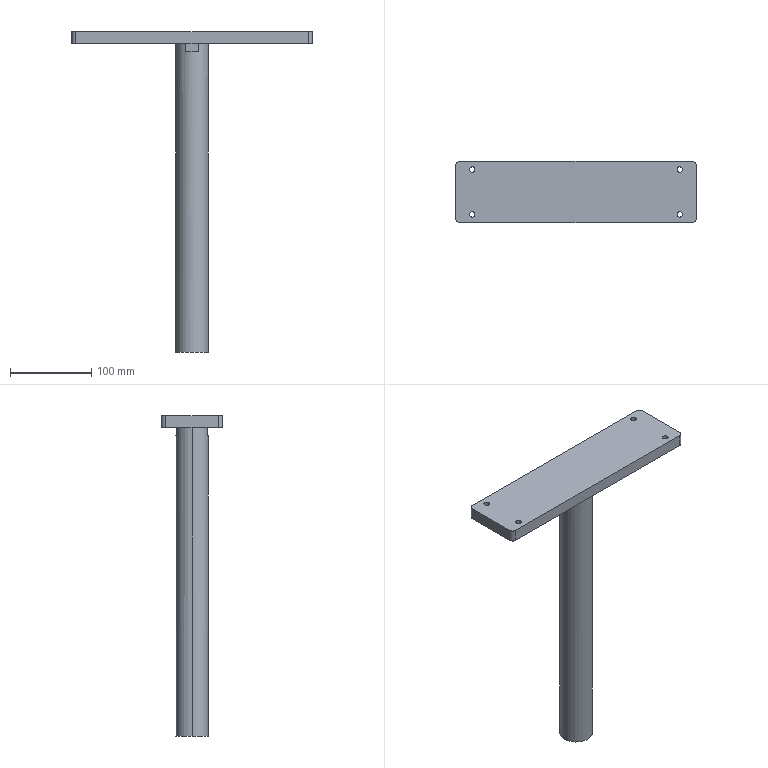Part | STEP file | Electric cylinder assembly 1 | 1 solid | 25 faces | box 295 x 75 x 394 mm | volume 805333 mm3 | cylinder 14 | plane 11 | commonest cylinder face diameters 6.8 x8 10 x4 40 x2
STEP:
#1=CARTESIAN_POINT('',(15.373,-48.431,607.5));
#2=VERTEX_POINT('',#1);
#3=CARTESIAN_POINT('',(2.972,-29.931,607.5));
#4=VERTEX_POINT('',#3);
#5=CARTESIAN_POINT('',(-4.627,-48.431,607.5));
#6=DIRECTION('',(0.,0.,1.));
#7=DIRECTION('',(1.,0.,0.));
#8=AXIS2_PLACEMENT_3D('',#5,#6,#7);
#9=CIRCLE('',#8,20.);
#10=EDGE_CURVE('',#2,#4,#9,.T.);
#11=ORIENTED_EDGE('',*,*,#10,.F.);
#12=CARTESIAN_POINT('',(15.373,-48.431,228.5));
#13=VERTEX_POINT('',#12);
#14=CARTESIAN_POINT('',(15.373,-48.431,580.5));
#15=DIRECTION('',(0.,0.,-1.));
#16=VECTOR('',#15,1000.);
#17=LINE('',#14,#16);
#18=EDGE_CURVE('',#2,#13,#17,.T.);
#19=ORIENTED_EDGE('',*,*,#18,.T.);
#20=CARTESIAN_POINT('',(-24.627,-48.431,228.5));
#21=VERTEX_POINT('',#20);
#22=CARTESIAN_POINT('',(-4.627,-48.431,228.5));
#23=DIRECTION('',(0.,0.,-1.));
#24=DIRECTION('',(-1.,0.,0.));
#25=AXIS2_PLACEMENT_3D('',#22,#23,#24);
#26=CIRCLE('',#25,20.);
#27=EDGE_CURVE('',#21,#13,#26,.T.);
#28=ORIENTED_EDGE('',*,*,#27,.F.);
#29=CARTESIAN_POINT('',(-24.627,-48.431,607.5));
#30=VERTEX_POINT('',#29);
#31=CARTESIAN_POINT('',(-24.627,-48.431,580.5));
#32=DIRECTION('',(0.,0.,-1.));
#33=VECTOR('',#32,1000.);
#34=LINE('',#31,#33);
#35=EDGE_CURVE('',#30,#21,#34,.T.);
#36=ORIENTED_EDGE('',*,*,#35,.F.);
#37=CARTESIAN_POINT('',(-12.227,-29.931,607.5));
#38=VERTEX_POINT('',#37);
#39=CARTESIAN_POINT('',(-4.627,-48.431,607.5));
#40=DIRECTION('',(0.,0.,1.));
#41=DIRECTION('',(1.,0.,0.));
#42=AXIS2_PLACEMENT_3D('',#39,#40,#41);
#43=CIRCLE('',#42,20.);
#44=EDGE_CURVE('',#38,#30,#43,.T.);
#45=ORIENTED_EDGE('',*,*,#44,.F.);
#46=CARTESIAN_POINT('',(-12.227,-29.931,597.5));
#47=VERTEX_POINT('',#46);
#48=CARTESIAN_POINT('',(-12.227,-29.931,607.5));
#49=DIRECTION('',(0.,0.,-1.));
#50=VECTOR('',#49,1000.);
#51=LINE('',#48,#50);
#52=EDGE_CURVE('',#38,#47,#51,.T.);
#53=ORIENTED_EDGE('',*,*,#52,.T.);
#54=CARTESIAN_POINT('',(2.972,-29.931,597.5));
#55=VERTEX_POINT('',#54);
#56=CARTESIAN_POINT('',(-4.627,-48.431,597.5));
#57=DIRECTION('',(0.,0.,-1.));
#58=DIRECTION('',(-1.,0.,0.));
#59=AXIS2_PLACEMENT_3D('',#56,#57,#58);
#60=CIRCLE('',#59,20.);
#61=EDGE_CURVE('',#47,#55,#60,.T.);
#62=ORIENTED_EDGE('',*,*,#61,.T.);
#63=CARTESIAN_POINT('',(2.972,-29.931,607.5));
#64=DIRECTION('',(0.,0.,1.));
#65=VECTOR('',#64,1000.);
#66=LINE('',#63,#65);
#67=EDGE_CURVE('',#55,#4,#66,.T.);
#68=ORIENTED_EDGE('',*,*,#67,.T.);
#69=EDGE_LOOP('',(#11,#19,#28,#36,#45,#53,#62,#68));
#70=FACE_OUTER_BOUND('',#69,.T.);
#71=CARTESIAN_POINT('',(-4.627,-48.431,580.5));
#72=DIRECTION('',(0.,0.,-1.));
#73=DIRECTION('',(-1.,0.,0.));
#74=AXIS2_PLACEMENT_3D('',#71,#72,#73);
#75=CYLINDRICAL_SURFACE('',#74,20.);
#76=ADVANCED_FACE('',(#70),#75,.T.);
#77=CARTESIAN_POINT('',(137.873,-85.931,622.5));
#78=VERTEX_POINT('',#77);
#79=CARTESIAN_POINT('',(142.873,-80.931,622.5));
#80=VERTEX_POINT('',#79);
#81=CARTESIAN_POINT('',(137.873,-80.931,622.5));
#82=DIRECTION('',(0.,0.,1.));
#83=DIRECTION('',(1.,0.,0.));
#84=AXIS2_PLACEMENT_3D('',#81,#82,#83);
#85=CIRCLE('',#84,5.);
#86=EDGE_CURVE('',#78,#80,#85,.T.);
#87=ORIENTED_EDGE('',*,*,#86,.F.);
#88=CARTESIAN_POINT('',(137.873,-85.931,607.5));
#89=VERTEX_POINT('',#88);
#90=CARTESIAN_POINT('',(137.873,-85.931,622.5));
#91=DIRECTION('',(0.,0.,1.));
#92=VECTOR('',#91,1000.);
#93=LINE('',#90,#92);
#94=EDGE_CURVE('',#89,#78,#93,.T.);
#95=ORIENTED_EDGE('',*,*,#94,.F.);
#96=CARTESIAN_POINT('',(142.873,-80.931,607.5));
#97=VERTEX_POINT('',#96);
#98=CARTESIAN_POINT('',(137.873,-80.931,607.5));
#99=DIRECTION('',(0.,0.,-1.));
#100=DIRECTION('',(1.,0.,0.));
#101=AXIS2_PLACEMENT_3D('',#98,#99,#100);
#102=CIRCLE('',#101,5.);
#103=EDGE_CURVE('',#97,#89,#102,.T.);
#104=ORIENTED_EDGE('',*,*,#103,.F.);
#105=CARTESIAN_POINT('',(142.873,-80.931,622.5));
#106=DIRECTION('',(0.,0.,-1.));
#107=VECTOR('',#106,1000.);
#108=LINE('',#105,#107);
#109=EDGE_CURVE('',#80,#97,#108,.T.);
#110=ORIENTED_EDGE('',*,*,#109,.F.);
#111=EDGE_LOOP('',(#87,#95,#104,#110));
#112=FACE_OUTER_BOUND('',#111,.T.);
#113=CARTESIAN_POINT('',(137.873,-80.931,622.5));
#114=DIRECTION('',(0.,0.,-1.));
#115=DIRECTION('',(-1.,0.,0.));
#116=AXIS2_PLACEMENT_3D('',#113,#114,#115);
#117=CYLINDRICAL_SURFACE('',#116,5.);
#118=ADVANCED_FACE('',(#112),#117,.T.);
#119=CARTESIAN_POINT('',(142.873,-15.931,607.5));
#120=VERTEX_POINT('',#119);
#121=CARTESIAN_POINT('',(142.873,-10.931,607.5));
#122=DIRECTION('',(0.,1.,0.));
#123=VECTOR('',#122,1000.);
#124=LINE('',#121,#123);
#125=EDGE_CURVE('',#97,#120,#124,.T.);
#126=ORIENTED_EDGE('',*,*,#125,.T.);
#127=CARTESIAN_POINT('',(142.873,-15.931,622.5));
#128=VERTEX_POINT('',#127);
#129=CARTESIAN_POINT('',(142.873,-15.931,622.5));
#130=DIRECTION('',(0.,0.,1.));
#131=VECTOR('',#130,1000.);
#132=LINE('',#129,#131);
#133=EDGE_CURVE('',#120,#128,#132,.T.);
#134=ORIENTED_EDGE('',*,*,#133,.T.);
#135=CARTESIAN_POINT('',(142.873,-10.931,622.5));
#136=DIRECTION('',(0.,1.,0.));
#137=VECTOR('',#136,1000.);
#138=LINE('',#135,#137);
#139=EDGE_CURVE('',#80,#128,#138,.T.);
#140=ORIENTED_EDGE('',*,*,#139,.F.);
#141=ORIENTED_EDGE('',*,*,#109,.T.);
#142=EDGE_LOOP('',(#126,#134,#140,#141));
#143=FACE_OUTER_BOUND('',#142,.T.);
#144=CARTESIAN_POINT('',(142.873,-10.931,622.5));
#145=DIRECTION('',(-1.,0.,0.));
#146=DIRECTION('',(0.,0.,1.));
#147=AXIS2_PLACEMENT_3D('',#144,#145,#146);
#148=PLANE('',#147);
#149=ADVANCED_FACE('',(#143),#148,.F.);
#150=CARTESIAN_POINT('',(137.873,-10.931,622.5));
#151=VERTEX_POINT('',#150);
#152=CARTESIAN_POINT('',(137.873,-15.931,622.5));
#153=DIRECTION('',(0.,0.,1.));
#154=DIRECTION('',(1.,0.,0.));
#155=AXIS2_PLACEMENT_3D('',#152,#153,#154);
#156=CIRCLE('',#155,5.);
#157=EDGE_CURVE('',#128,#151,#156,.T.);
#158=ORIENTED_EDGE('',*,*,#157,.F.);
#159=ORIENTED_EDGE('',*,*,#133,.F.);
#160=CARTESIAN_POINT('',(137.873,-10.931,607.5));
#161=VERTEX_POINT('',#160);
#162=CARTESIAN_POINT('',(137.873,-15.931,607.5));
#163=DIRECTION('',(0.,0.,-1.));
#164=DIRECTION('',(1.,0.,0.));
#165=AXIS2_PLACEMENT_3D('',#162,#163,#164);
#166=CIRCLE('',#165,5.);
#167=EDGE_CURVE('',#161,#120,#166,.T.);
#168=ORIENTED_EDGE('',*,*,#167,.F.);
#169=CARTESIAN_POINT('',(137.873,-10.931,622.5));
#170=DIRECTION('',(0.,0.,-1.));
#171=VECTOR('',#170,1000.);
#172=LINE('',#169,#171);
#173=EDGE_CURVE('',#151,#161,#172,.T.);
#174=ORIENTED_EDGE('',*,*,#173,.F.);
#175=EDGE_LOOP('',(#158,#159,#168,#174));
#176=FACE_OUTER_BOUND('',#175,.T.);
#177=CARTESIAN_POINT('',(137.873,-15.931,622.5));
#178=DIRECTION('',(0.,0.,-1.));
#179=DIRECTION('',(-1.,0.,0.));
#180=AXIS2_PLACEMENT_3D('',#177,#178,#179);
#181=CYLINDRICAL_SURFACE('',#180,5.);
#182=ADVANCED_FACE('',(#176),#181,.T.);
#183=CARTESIAN_POINT('',(119.473,-20.931,607.5));
#184=VERTEX_POINT('',#183);
#185=CARTESIAN_POINT('',(126.273,-20.931,607.5));
#186=VERTEX_POINT('',#185);
#187=CARTESIAN_POINT('',(122.873,-20.931,607.5));
#188=DIRECTION('',(0.,0.,1.));
#189=DIRECTION('',(1.,0.,0.));
#190=AXIS2_PLACEMENT_3D('',#187,#188,#189);
#191=CIRCLE('',#190,3.4);
#192=EDGE_CURVE('',#184,#186,#191,.T.);
#193=ORIENTED_EDGE('',*,*,#192,.F.);
#194=CARTESIAN_POINT('',(119.473,-20.931,622.5));
#195=VERTEX_POINT('',#194);
#196=CARTESIAN_POINT('',(119.473,-20.931,622.5));
#197=DIRECTION('',(0.,0.,1.));
#198=VECTOR('',#197,1000.);
#199=LINE('',#196,#198);
#200=EDGE_CURVE('',#184,#195,#199,.T.);
#201=ORIENTED_EDGE('',*,*,#200,.T.);
#202=CARTESIAN_POINT('',(126.273,-20.931,622.5));
#203=VERTEX_POINT('',#202);
#204=CARTESIAN_POINT('',(122.873,-20.931,622.5));
#205=DIRECTION('',(0.,0.,1.));
#206=DIRECTION('',(1.,0.,0.));
#207=AXIS2_PLACEMENT_3D('',#204,#205,#206);
#208=CIRCLE('',#207,3.4);
#209=EDGE_CURVE('',#195,#203,#208,.T.);
#210=ORIENTED_EDGE('',*,*,#209,.T.);
#211=CARTESIAN_POINT('',(126.273,-20.931,622.5));
#212=DIRECTION('',(0.,0.,1.));
#213=VECTOR('',#212,1000.);
#214=LINE('',#211,#213);
#215=EDGE_CURVE('',#186,#203,#214,.T.);
#216=ORIENTED_EDGE('',*,*,#215,.F.);
#217=EDGE_LOOP('',(#193,#201,#210,#216));
#218=FACE_OUTER_BOUND('',#217,.T.);
#219=CARTESIAN_POINT('',(122.873,-20.931,622.5));
#220=DIRECTION('',(0.,0.,1.));
#221=DIRECTION('',(1.,0.,0.));
#222=AXIS2_PLACEMENT_3D('',#219,#220,#221);
#223=CYLINDRICAL_SURFACE('',#222,3.4);
#224=ADVANCED_FACE('',(#218),#223,.F.);
#225=ORIENTED_EDGE('',*,*,#200,.F.);
#226=CARTESIAN_POINT('',(122.873,-20.931,607.5));
#227=DIRECTION('',(0.,0.,1.));
#228=DIRECTION('',(1.,0.,0.));
#229=AXIS2_PLACEMENT_3D('',#226,#227,#228);
#230=CIRCLE('',#229,3.4);
#231=EDGE_CURVE('',#186,#184,#230,.T.);
#232=ORIENTED_EDGE('',*,*,#231,.F.);
#233=ORIENTED_EDGE('',*,*,#215,.T.);
#234=CARTESIAN_POINT('',(122.873,-20.931,622.5));
#235=DIRECTION('',(0.,0.,1.));
#236=DIRECTION('',(1.,0.,0.));
#237=AXIS2_PLACEMENT_3D('',#234,#235,#236);
#238=CIRCLE('',#237,3.4);
#239=EDGE_CURVE('',#203,#195,#238,.T.);
#240=ORIENTED_EDGE('',*,*,#239,.T.);
#241=EDGE_LOOP('',(#225,#232,#233,#240));
#242=FACE_OUTER_BOUND('',#241,.T.);
#243=CARTESIAN_POINT('',(122.873,-20.931,622.5));
#244=DIRECTION('',(0.,0.,1.));
#245=DIRECTION('',(1.,0.,0.));
#246=AXIS2_PLACEMENT_3D('',#243,#244,#245);
#247=CYLINDRICAL_SURFACE('',#246,3.4);
#248=ADVANCED_FACE('',(#242),#247,.F.);
#249=CARTESIAN_POINT('',(119.473,-75.931,607.5));
#250=VERTEX_POINT('',#249);
#251=CARTESIAN_POINT('',(126.273,-75.931,607.5));
#252=VERTEX_POINT('',#251);
#253=CARTESIAN_POINT('',(122.873,-75.931,607.5));
#254=DIRECTION('',(0.,0.,1.));
#255=DIRECTION('',(1.,0.,0.));
#256=AXIS2_PLACEMENT_3D('',#253,#254,#255);
#257=CIRCLE('',#256,3.4);
#258=EDGE_CURVE('',#250,#252,#257,.T.);
#259=ORIENTED_EDGE('',*,*,#258,.F.);
#260=CARTESIAN_POINT('',(119.473,-75.931,622.5));
#261=VERTEX_POINT('',#260);
#262=CARTESIAN_POINT('',(119.473,-75.931,622.5));
#263=DIRECTION('',(0.,0.,1.));
#264=VECTOR('',#263,1000.);
#265=LINE('',#262,#264);
#266=EDGE_CURVE('',#250,#261,#265,.T.);
#267=ORIENTED_EDGE('',*,*,#266,.T.);
#268=CARTESIAN_POINT('',(126.273,-75.931,622.5));
#269=VERTEX_POINT('',#268);
#270=CARTESIAN_POINT('',(122.873,-75.931,622.5));
#271=DIRECTION('',(0.,0.,1.));
#272=DIRECTION('',(1.,0.,0.));
#273=AXIS2_PLACEMENT_3D('',#270,#271,#272);
#274=CIRCLE('',#273,3.4);
#275=EDGE_CURVE('',#261,#269,#274,.T.);
#276=ORIENTED_EDGE('',*,*,#275,.T.);
#277=CARTESIAN_POINT('',(126.273,-75.931,622.5));
#278=DIRECTION('',(0.,0.,1.));
#279=VECTOR('',#278,1000.);
#280=LINE('',#277,#279);
#281=EDGE_CURVE('',#252,#269,#280,.T.);
#282=ORIENTED_EDGE('',*,*,#281,.F.);
#283=EDGE_LOOP('',(#259,#267,#276,#282));
#284=FACE_OUTER_BOUND('',#283,.T.);
#285=CARTESIAN_POINT('',(122.873,-75.931,622.5));
#286=DIRECTION('',(0.,0.,1.));
#287=DIRECTION('',(1.,0.,0.));
#288=AXIS2_PLACEMENT_3D('',#285,#286,#287);
#289=CYLINDRICAL_SURFACE('',#288,3.4);
#290=ADVANCED_FACE('',(#284),#289,.F.);
#291=ORIENTED_EDGE('',*,*,#266,.F.);
#292=CARTESIAN_POINT('',(122.873,-75.931,607.5));
#293=DIRECTION('',(0.,0.,1.));
#294=DIRECTION('',(1.,0.,0.));
#295=AXIS2_PLACEMENT_3D('',#292,#293,#294);
#296=CIRCLE('',#295,3.4);
#297=EDGE_CURVE('',#252,#250,#296,.T.);
#298=ORIENTED_EDGE('',*,*,#297,.F.);
#299=ORIENTED_EDGE('',*,*,#281,.T.);
#300=CARTESIAN_POINT('',(122.873,-75.931,622.5));
#301=DIRECTION('',(0.,0.,1.));
#302=DIRECTION('',(1.,0.,0.));
#303=AXIS2_PLACEMENT_3D('',#300,#301,#302);
#304=CIRCLE('',#303,3.4);
#305=EDGE_CURVE('',#269,#261,#304,.T.);
#306=ORIENTED_EDGE('',*,*,#305,.T.);
#307=EDGE_LOOP('',(#291,#298,#299,#306));
#308=FACE_OUTER_BOUND('',#307,.T.);
#309=CARTESIAN_POINT('',(122.873,-75.931,622.5));
#310=DIRECTION('',(0.,0.,1.));
#311=DIRECTION('',(1.,0.,0.));
#312=AXIS2_PLACEMENT_3D('',#309,#310,#311);
#313=CYLINDRICAL_SURFACE('',#312,3.4);
#314=ADVANCED_FACE('',(#308),#313,.F.);
#315=ORIENTED_EDGE('',*,*,#297,.T.);
#316=ORIENTED_EDGE('',*,*,#258,.T.);
#317=EDGE_LOOP('',(#315,#316));
#318=FACE_BOUND('',#317,.T.);
#319=ORIENTED_EDGE('',*,*,#231,.T.);
#320=ORIENTED_EDGE('',*,*,#192,.T.);
#321=EDGE_LOOP('',(#319,#320));
#322=FACE_BOUND('',#321,.T.);
#323=CARTESIAN_POINT('',(-147.127,-85.931,607.5));
#324=VERTEX_POINT('',#323);
#325=CARTESIAN_POINT('',(-12.127,-85.931,607.5));
#326=DIRECTION('',(1.,0.,0.));
#327=VECTOR('',#326,1000.);
#328=LINE('',#325,#327);
#329=EDGE_CURVE('',#324,#89,#328,.T.);
#330=ORIENTED_EDGE('',*,*,#329,.F.);
#331=CARTESIAN_POINT('',(-152.127,-80.931,607.5));
#332=VERTEX_POINT('',#331);
#333=CARTESIAN_POINT('',(-147.127,-80.931,607.5));
#334=DIRECTION('',(0.,0.,-1.));
#335=DIRECTION('',(1.,0.,0.));
#336=AXIS2_PLACEMENT_3D('',#333,#334,#335);
#337=CIRCLE('',#336,5.);
#338=EDGE_CURVE('',#324,#332,#337,.T.);
#339=ORIENTED_EDGE('',*,*,#338,.T.);
#340=CARTESIAN_POINT('',(-152.127,-15.931,607.5));
#341=VERTEX_POINT('',#340);
#342=CARTESIAN_POINT('',(-152.127,-10.931,607.5));
#343=DIRECTION('',(0.,-1.,0.));
#344=VECTOR('',#343,1000.);
#345=LINE('',#342,#344);
#346=EDGE_CURVE('',#341,#332,#345,.T.);
#347=ORIENTED_EDGE('',*,*,#346,.F.);
#348=CARTESIAN_POINT('',(-147.127,-10.931,607.5));
#349=VERTEX_POINT('',#348);
#350=CARTESIAN_POINT('',(-147.127,-15.931,607.5));
#351=DIRECTION('',(0.,0.,-1.));
#352=DIRECTION('',(1.,0.,0.));
#353=AXIS2_PLACEMENT_3D('',#350,#351,#352);
#354=CIRCLE('',#353,5.);
#355=EDGE_CURVE('',#341,#349,#354,.T.);
#356=ORIENTED_EDGE('',*,*,#355,.T.);
#357=CARTESIAN_POINT('',(-12.127,-10.931,607.5));
#358=DIRECTION('',(-1.,0.,0.));
#359=VECTOR('',#358,1000.);
#360=LINE('',#357,#359);
#361=EDGE_CURVE('',#161,#349,#360,.T.);
#362=ORIENTED_EDGE('',*,*,#361,.F.);
#363=ORIENTED_EDGE('',*,*,#167,.T.);
#364=ORIENTED_EDGE('',*,*,#125,.F.);
#365=ORIENTED_EDGE('',*,*,#103,.T.);
#366=EDGE_LOOP('',(#330,#339,#347,#356,#362,#363,#364,#365));
#367=FACE_OUTER_BOUND('',#366,.T.);
#368=CARTESIAN_POINT('',(2.972,-66.931,607.5));
#369=VERTEX_POINT('',#368);
#370=CARTESIAN_POINT('',(-4.627,-48.431,607.5));
#371=DIRECTION('',(0.,0.,1.));
#372=DIRECTION('',(1.,0.,0.));
#373=AXIS2_PLACEMENT_3D('',#370,#371,#372);
#374=CIRCLE('',#373,20.);
#375=EDGE_CURVE('',#369,#2,#374,.T.);
#376=ORIENTED_EDGE('',*,*,#375,.T.);
#377=ORIENTED_EDGE('',*,*,#10,.T.);
#378=CARTESIAN_POINT('',(-4.627,-29.931,607.5));
#379=DIRECTION('',(1.,0.,0.));
#380=VECTOR('',#379,1000.);
#381=LINE('',#378,#380);
#382=EDGE_CURVE('',#38,#4,#381,.T.);
#383=ORIENTED_EDGE('',*,*,#382,.F.);
#384=ORIENTED_EDGE('',*,*,#44,.T.);
#385=CARTESIAN_POINT('',(-12.227,-66.931,607.5));
#386=VERTEX_POINT('',#385);
#387=CARTESIAN_POINT('',(-4.627,-48.431,607.5));
#388=DIRECTION('',(0.,0.,1.));
#389=DIRECTION('',(1.,0.,0.));
#390=AXIS2_PLACEMENT_3D('',#387,#388,#389);
#391=CIRCLE('',#390,20.);
#392=EDGE_CURVE('',#30,#386,#391,.T.);
#393=ORIENTED_EDGE('',*,*,#392,.T.);
#394=CARTESIAN_POINT('',(-4.627,-66.931,607.5));
#395=DIRECTION('',(-1.,0.,0.));
#396=VECTOR('',#395,1000.);
#397=LINE('',#394,#396);
#398=EDGE_CURVE('',#369,#386,#397,.T.);
#399=ORIENTED_EDGE('',*,*,#398,.F.);
#400=EDGE_LOOP('',(#376,#377,#383,#384,#393,#399));
#401=FACE_BOUND('',#400,.T.);
#402=CARTESIAN_POINT('',(-128.727,-75.931,607.5));
#403=VERTEX_POINT('',#402);
#404=CARTESIAN_POINT('',(-135.527,-75.931,607.5));
#405=VERTEX_POINT('',#404);
#406=CARTESIAN_POINT('',(-132.127,-75.931,607.5));
#407=DIRECTION('',(0.,0.,1.));
#408=DIRECTION('',(1.,0.,0.));
#409=AXIS2_PLACEMENT_3D('',#406,#407,#408);
#410=CIRCLE('',#409,3.4);
#411=EDGE_CURVE('',#403,#405,#410,.T.);
#412=ORIENTED_EDGE('',*,*,#411,.T.);
#413=CARTESIAN_POINT('',(-132.127,-75.931,607.5));
#414=DIRECTION('',(0.,0.,1.));
#415=DIRECTION('',(1.,0.,0.));
#416=AXIS2_PLACEMENT_3D('',#413,#414,#415);
#417=CIRCLE('',#416,3.4);
#418=EDGE_CURVE('',#405,#403,#417,.T.);
#419=ORIENTED_EDGE('',*,*,#418,.T.);
#420=EDGE_LOOP('',(#412,#419));
#421=FACE_BOUND('',#420,.T.);
#422=CARTESIAN_POINT('',(-128.727,-20.931,607.5));
#423=VERTEX_POINT('',#422);
#424=CARTESIAN_POINT('',(-135.527,-20.931,607.5));
#425=VERTEX_POINT('',#424);
#426=CARTESIAN_POINT('',(-132.127,-20.931,607.5));
#427=DIRECTION('',(0.,0.,1.));
#428=DIRECTION('',(1.,0.,0.));
#429=AXIS2_PLACEMENT_3D('',#426,#427,#428);
#430=CIRCLE('',#429,3.4);
#431=EDGE_CURVE('',#423,#425,#430,.T.);
#432=ORIENTED_EDGE('',*,*,#431,.T.);
#433=CARTESIAN_POINT('',(-132.127,-20.931,607.5));
#434=DIRECTION('',(0.,0.,1.));
#435=DIRECTION('',(1.,0.,0.));
#436=AXIS2_PLACEMENT_3D('',#433,#434,#435);
#437=CIRCLE('',#436,3.4);
#438=EDGE_CURVE('',#425,#423,#437,.T.);
#439=ORIENTED_EDGE('',*,*,#438,.T.);
#440=EDGE_LOOP('',(#432,#439));
#441=FACE_BOUND('',#440,.T.);
#442=CARTESIAN_POINT('',(65.373,-48.431,607.5));
#443=DIRECTION('',(0.,0.,1.));
#444=DIRECTION('',(1.,0.,0.));
#445=AXIS2_PLACEMENT_3D('',#442,#443,#444);
#446=PLANE('',#445);
#447=ADVANCED_FACE('',(#318,#322,#367,#401,#421,#441),#446,.F.);
#448=ORIENTED_EDGE('',*,*,#361,.T.);
#449=CARTESIAN_POINT('',(-147.127,-10.931,622.5));
#450=VERTEX_POINT('',#449);
#451=CARTESIAN_POINT('',(-147.127,-10.931,622.5));
#452=DIRECTION('',(0.,0.,1.));
#453=VECTOR('',#452,1000.);
#454=LINE('',#451,#453);
#455=EDGE_CURVE('',#349,#450,#454,.T.);
#456=ORIENTED_EDGE('',*,*,#455,.T.);
#457=CARTESIAN_POINT('',(-12.127,-10.931,622.5));
#458=DIRECTION('',(-1.,0.,0.));
#459=VECTOR('',#458,1000.);
#460=LINE('',#457,#459);
#461=EDGE_CURVE('',#151,#450,#460,.T.);
#462=ORIENTED_EDGE('',*,*,#461,.F.);
#463=ORIENTED_EDGE('',*,*,#173,.T.);
#464=EDGE_LOOP('',(#448,#456,#462,#463));
#465=FACE_OUTER_BOUND('',#464,.T.);
#466=CARTESIAN_POINT('',(-12.127,-10.931,622.5));
#467=DIRECTION('',(0.,-1.,0.));
#468=DIRECTION('',(0.,0.,-1.));
#469=AXIS2_PLACEMENT_3D('',#466,#467,#468);
#470=PLANE('',#469);
#471=ADVANCED_FACE('',(#465),#470,.F.);
#472=CARTESIAN_POINT('',(-147.127,-85.931,622.5));
#473=VERTEX_POINT('',#472);
#474=CARTESIAN_POINT('',(-12.127,-85.931,622.5));
#475=DIRECTION('',(1.,0.,0.));
#476=VECTOR('',#475,1000.);
#477=LINE('',#474,#476);
#478=EDGE_CURVE('',#473,#78,#477,.T.);
#479=ORIENTED_EDGE('',*,*,#478,.F.);
#480=CARTESIAN_POINT('',(-147.127,-85.931,622.5));
#481=DIRECTION('',(0.,0.,-1.));
#482=VECTOR('',#481,1000.);
#483=LINE('',#480,#482);
#484=EDGE_CURVE('',#473,#324,#483,.T.);
#485=ORIENTED_EDGE('',*,*,#484,.T.);
#486=ORIENTED_EDGE('',*,*,#329,.T.);
#487=ORIENTED_EDGE('',*,*,#94,.T.);
#488=EDGE_LOOP('',(#479,#485,#486,#487));
#489=FACE_OUTER_BOUND('',#488,.T.);
#490=CARTESIAN_POINT('',(-12.127,-85.931,622.5));
#491=DIRECTION('',(0.,1.,0.));
#492=DIRECTION('',(1.,0.,0.));
#493=AXIS2_PLACEMENT_3D('',#490,#491,#492);
#494=PLANE('',#493);
#495=ADVANCED_FACE('',(#489),#494,.F.);
#496=ORIENTED_EDGE('',*,*,#461,.T.);
#497=CARTESIAN_POINT('',(-152.127,-15.931,622.5));
#498=VERTEX_POINT('',#497);
#499=CARTESIAN_POINT('',(-147.127,-15.931,622.5));
#500=DIRECTION('',(0.,0.,1.));
#501=DIRECTION('',(1.,0.,0.));
#502=AXIS2_PLACEMENT_3D('',#499,#500,#501);
#503=CIRCLE('',#502,5.);
#504=EDGE_CURVE('',#450,#498,#503,.T.);
#505=ORIENTED_EDGE('',*,*,#504,.T.);
#506=CARTESIAN_POINT('',(-152.127,-80.931,622.5));
#507=VERTEX_POINT('',#506);
#508=CARTESIAN_POINT('',(-152.127,-10.931,622.5));
#509=DIRECTION('',(0.,-1.,0.));
#510=VECTOR('',#509,1000.);
#511=LINE('',#508,#510);
#512=EDGE_CURVE('',#498,#507,#511,.T.);
#513=ORIENTED_EDGE('',*,*,#512,.T.);
#514=CARTESIAN_POINT('',(-147.127,-80.931,622.5));
#515=DIRECTION('',(0.,0.,1.));
#516=DIRECTION('',(1.,0.,0.));
#517=AXIS2_PLACEMENT_3D('',#514,#515,#516);
#518=CIRCLE('',#517,5.);
#519=EDGE_CURVE('',#507,#473,#518,.T.);
#520=ORIENTED_EDGE('',*,*,#519,.T.);
#521=ORIENTED_EDGE('',*,*,#478,.T.);
#522=ORIENTED_EDGE('',*,*,#86,.T.);
#523=ORIENTED_EDGE('',*,*,#139,.T.);
#524=ORIENTED_EDGE('',*,*,#157,.T.);
#525=EDGE_LOOP('',(#496,#505,#513,#520,#521,#522,#523,#524));
#526=FACE_OUTER_BOUND('',#525,.T.);
#527=ORIENTED_EDGE('',*,*,#305,.F.);
#528=ORIENTED_EDGE('',*,*,#275,.F.);
#529=EDGE_LOOP('',(#527,#528));
#530=FACE_BOUND('',#529,.T.);
#531=ORIENTED_EDGE('',*,*,#239,.F.);
#532=ORIENTED_EDGE('',*,*,#209,.F.);
#533=EDGE_LOOP('',(#531,#532));
#534=FACE_BOUND('',#533,.T.);
#535=CARTESIAN_POINT('',(-128.727,-20.931,622.5));
#536=VERTEX_POINT('',#535);
#537=CARTESIAN_POINT('',(-135.527,-20.931,622.5));
#538=VERTEX_POINT('',#537);
#539=CARTESIAN_POINT('',(-132.127,-20.931,622.5));
#540=DIRECTION('',(0.,0.,1.));
#541=DIRECTION('',(1.,0.,0.));
#542=AXIS2_PLACEMENT_3D('',#539,#540,#541);
#543=CIRCLE('',#542,3.4);
#544=EDGE_CURVE('',#536,#538,#543,.T.);
#545=ORIENTED_EDGE('',*,*,#544,.F.);
#546=CARTESIAN_POINT('',(-132.127,-20.931,622.5));
#547=DIRECTION('',(0.,0.,1.));
#548=DIRECTION('',(1.,0.,0.));
#549=AXIS2_PLACEMENT_3D('',#546,#547,#548);
#550=CIRCLE('',#549,3.4);
#551=EDGE_CURVE('',#538,#536,#550,.T.);
#552=ORIENTED_EDGE('',*,*,#551,.F.);
#553=EDGE_LOOP('',(#545,#552));
#554=FACE_BOUND('',#553,.T.);
#555=CARTESIAN_POINT('',(-128.727,-75.931,622.5));
#556=VERTEX_POINT('',#555);
#557=CARTESIAN_POINT('',(-135.527,-75.931,622.5));
#558=VERTEX_POINT('',#557);
#559=CARTESIAN_POINT('',(-132.127,-75.931,622.5));
#560=DIRECTION('',(0.,0.,1.));
#561=DIRECTION('',(1.,0.,0.));
#562=AXIS2_PLACEMENT_3D('',#559,#560,#561);
#563=CIRCLE('',#562,3.4);
#564=EDGE_CURVE('',#556,#558,#563,.T.);
#565=ORIENTED_EDGE('',*,*,#564,.F.);
#566=CARTESIAN_POINT('',(-132.127,-75.931,622.5));
#567=DIRECTION('',(0.,0.,1.));
#568=DIRECTION('',(1.,0.,0.));
#569=AXIS2_PLACEMENT_3D('',#566,#567,#568);
#570=CIRCLE('',#569,3.4);
#571=EDGE_CURVE('',#558,#556,#570,.T.);
#572=ORIENTED_EDGE('',*,*,#571,.F.);
#573=EDGE_LOOP('',(#565,#572));
#574=FACE_BOUND('',#573,.T.);
#575=CARTESIAN_POINT('',(65.373,-48.431,622.5));
#576=DIRECTION('',(0.,0.,1.));
#577=DIRECTION('',(1.,0.,0.));
#578=AXIS2_PLACEMENT_3D('',#575,#576,#577);
#579=PLANE('',#578);
#580=ADVANCED_FACE('',(#526,#530,#534,#554,#574),#579,.T.);
#581=ORIENTED_EDGE('',*,*,#18,.F.);
#582=ORIENTED_EDGE('',*,*,#375,.F.);
#583=CARTESIAN_POINT('',(2.972,-66.931,597.5));
#584=VERTEX_POINT('',#583);
#585=CARTESIAN_POINT('',(2.972,-66.931,607.5));
#586=DIRECTION('',(0.,0.,-1.));
#587=VECTOR('',#586,1000.);
#588=LINE('',#585,#587);
#589=EDGE_CURVE('',#369,#584,#588,.T.);
#590=ORIENTED_EDGE('',*,*,#589,.T.);
#591=CARTESIAN_POINT('',(-12.227,-66.931,597.5));
#592=VERTEX_POINT('',#591);
#593=CARTESIAN_POINT('',(-4.627,-48.431,597.5));
#594=DIRECTION('',(0.,0.,-1.));
#595=DIRECTION('',(-1.,0.,0.));
#596=AXIS2_PLACEMENT_3D('',#593,#594,#595);
#597=CIRCLE('',#596,20.);
#598=EDGE_CURVE('',#584,#592,#597,.T.);
#599=ORIENTED_EDGE('',*,*,#598,.T.);
#600=CARTESIAN_POINT('',(-12.227,-66.931,607.5));
#601=DIRECTION('',(0.,0.,1.));
#602=VECTOR('',#601,1000.);
#603=LINE('',#600,#602);
#604=EDGE_CURVE('',#592,#386,#603,.T.);
#605=ORIENTED_EDGE('',*,*,#604,.T.);
#606=ORIENTED_EDGE('',*,*,#392,.F.);
#607=ORIENTED_EDGE('',*,*,#35,.T.);
#608=CARTESIAN_POINT('',(-4.627,-48.431,228.5));
#609=DIRECTION('',(0.,0.,-1.));
#610=DIRECTION('',(-1.,0.,0.));
#611=AXIS2_PLACEMENT_3D('',#608,#609,#610);
#612=CIRCLE('',#611,20.);
#613=EDGE_CURVE('',#13,#21,#612,.T.);
#614=ORIENTED_EDGE('',*,*,#613,.F.);
#615=EDGE_LOOP('',(#581,#582,#590,#599,#605,#606,#607,#614));
#616=FACE_OUTER_BOUND('',#615,.T.);
#617=CARTESIAN_POINT('',(-4.627,-48.431,580.5));
#618=DIRECTION('',(0.,0.,-1.));
#619=DIRECTION('',(-1.,0.,0.));
#620=AXIS2_PLACEMENT_3D('',#617,#618,#619);
#621=CYLINDRICAL_SURFACE('',#620,20.);
#622=ADVANCED_FACE('',(#616),#621,.T.);
#623=CARTESIAN_POINT('',(-82.127,-29.931,597.5));
#624=DIRECTION('',(1.,0.,0.));
#625=VECTOR('',#624,1000.);
#626=LINE('',#623,#625);
#627=EDGE_CURVE('',#47,#55,#626,.T.);
#628=ORIENTED_EDGE('',*,*,#627,.T.);
#629=ORIENTED_EDGE('',*,*,#61,.F.);
#630=EDGE_LOOP('',(#628,#629));
#631=FACE_OUTER_BOUND('',#630,.T.);
#632=CARTESIAN_POINT('',(-82.127,-16.958,597.5));
#633=DIRECTION('',(0.,0.,-1.));
#634=DIRECTION('',(0.,-1.,0.));
#635=AXIS2_PLACEMENT_3D('',#632,#633,#634);
#636=PLANE('',#635);
#637=ADVANCED_FACE('',(#631),#636,.F.);
#638=ORIENTED_EDGE('',*,*,#382,.T.);
#639=ORIENTED_EDGE('',*,*,#67,.F.);
#640=ORIENTED_EDGE('',*,*,#627,.F.);
#641=ORIENTED_EDGE('',*,*,#52,.F.);
#642=EDGE_LOOP('',(#638,#639,#640,#641));
#643=FACE_OUTER_BOUND('',#642,.T.);
#644=CARTESIAN_POINT('',(-82.127,-29.931,615.257));
#645=DIRECTION('',(0.,-1.,0.));
#646=DIRECTION('',(0.,0.,-1.));
#647=AXIS2_PLACEMENT_3D('',#644,#645,#646);
#648=PLANE('',#647);
#649=ADVANCED_FACE('',(#643),#648,.F.);
#650=CARTESIAN_POINT('',(-82.127,-66.931,597.5));
#651=DIRECTION('',(1.,0.,0.));
#652=VECTOR('',#651,1000.);
#653=LINE('',#650,#652);
#654=EDGE_CURVE('',#592,#584,#653,.T.);
#655=ORIENTED_EDGE('',*,*,#654,.F.);
#656=ORIENTED_EDGE('',*,*,#598,.F.);
#657=EDGE_LOOP('',(#655,#656));
#658=FACE_OUTER_BOUND('',#657,.T.);
#659=CARTESIAN_POINT('',(-82.127,-79.904,597.5));
#660=DIRECTION('',(0.,0.,-1.));
#661=DIRECTION('',(0.,-1.,0.));
#662=AXIS2_PLACEMENT_3D('',#659,#660,#661);
#663=PLANE('',#662);
#664=ADVANCED_FACE('',(#658),#663,.F.);
#665=ORIENTED_EDGE('',*,*,#398,.T.);
#666=ORIENTED_EDGE('',*,*,#604,.F.);
#667=ORIENTED_EDGE('',*,*,#654,.T.);
#668=ORIENTED_EDGE('',*,*,#589,.F.);
#669=EDGE_LOOP('',(#665,#666,#667,#668));
#670=FACE_OUTER_BOUND('',#669,.T.);
#671=CARTESIAN_POINT('',(-82.127,-66.931,615.257));
#672=DIRECTION('',(0.,1.,0.));
#673=DIRECTION('',(0.,0.,-1.));
#674=AXIS2_PLACEMENT_3D('',#671,#672,#673);
#675=PLANE('',#674);
#676=ADVANCED_FACE('',(#670),#675,.F.);
#677=ORIENTED_EDGE('',*,*,#27,.T.);
#678=ORIENTED_EDGE('',*,*,#613,.T.);
#679=EDGE_LOOP('',(#677,#678));
#680=FACE_OUTER_BOUND('',#679,.T.);
#681=CARTESIAN_POINT('',(-4.627,-48.431,228.5));
#682=DIRECTION('',(0.,0.,-1.));
#683=DIRECTION('',(-1.,0.,0.));
#684=AXIS2_PLACEMENT_3D('',#681,#682,#683);
#685=PLANE('',#684);
#686=ADVANCED_FACE('',(#680),#685,.T.);
#687=ORIENTED_EDGE('',*,*,#504,.F.);
#688=ORIENTED_EDGE('',*,*,#455,.F.);
#689=ORIENTED_EDGE('',*,*,#355,.F.);
#690=CARTESIAN_POINT('',(-152.127,-15.931,622.5));
#691=DIRECTION('',(0.,0.,-1.));
#692=VECTOR('',#691,1000.);
#693=LINE('',#690,#692);
#694=EDGE_CURVE('',#498,#341,#693,.T.);
#695=ORIENTED_EDGE('',*,*,#694,.F.);
#696=EDGE_LOOP('',(#687,#688,#689,#695));
#697=FACE_OUTER_BOUND('',#696,.T.);
#698=CARTESIAN_POINT('',(-147.127,-15.931,622.5));
#699=DIRECTION('',(0.,0.,-1.));
#700=DIRECTION('',(-1.,0.,0.));
#701=AXIS2_PLACEMENT_3D('',#698,#699,#700);
#702=CYLINDRICAL_SURFACE('',#701,5.);
#703=ADVANCED_FACE('',(#697),#702,.T.);
#704=ORIENTED_EDGE('',*,*,#512,.F.);
#705=ORIENTED_EDGE('',*,*,#694,.T.);
#706=ORIENTED_EDGE('',*,*,#346,.T.);
#707=CARTESIAN_POINT('',(-152.127,-80.931,622.5));
#708=DIRECTION('',(0.,0.,1.));
#709=VECTOR('',#708,1000.);
#710=LINE('',#707,#709);
#711=EDGE_CURVE('',#332,#507,#710,.T.);
#712=ORIENTED_EDGE('',*,*,#711,.T.);
#713=EDGE_LOOP('',(#704,#705,#706,#712));
#714=FACE_OUTER_BOUND('',#713,.T.);
#715=CARTESIAN_POINT('',(-152.127,-10.931,622.5));
#716=DIRECTION('',(1.,0.,0.));
#717=DIRECTION('',(0.,1.,0.));
#718=AXIS2_PLACEMENT_3D('',#715,#716,#717);
#719=PLANE('',#718);
#720=ADVANCED_FACE('',(#714),#719,.F.);
#721=ORIENTED_EDGE('',*,*,#519,.F.);
#722=ORIENTED_EDGE('',*,*,#711,.F.);
#723=ORIENTED_EDGE('',*,*,#338,.F.);
#724=ORIENTED_EDGE('',*,*,#484,.F.);
#725=EDGE_LOOP('',(#721,#722,#723,#724));
#726=FACE_OUTER_BOUND('',#725,.T.);
#727=CARTESIAN_POINT('',(-147.127,-80.931,622.5));
#728=DIRECTION('',(0.,0.,-1.));
#729=DIRECTION('',(-1.,0.,0.));
#730=AXIS2_PLACEMENT_3D('',#727,#728,#729);
#731=CYLINDRICAL_SURFACE('',#730,5.);
#732=ADVANCED_FACE('',(#726),#731,.T.);
#733=ORIENTED_EDGE('',*,*,#438,.F.);
#734=CARTESIAN_POINT('',(-135.527,-20.931,622.5));
#735=DIRECTION('',(0.,0.,1.));
#736=VECTOR('',#735,1000.);
#737=LINE('',#734,#736);
#738=EDGE_CURVE('',#425,#538,#737,.T.);
#739=ORIENTED_EDGE('',*,*,#738,.T.);
#740=ORIENTED_EDGE('',*,*,#551,.T.);
#741=CARTESIAN_POINT('',(-128.727,-20.931,622.5));
#742=DIRECTION('',(0.,0.,1.));
#743=VECTOR('',#742,1000.);
#744=LINE('',#741,#743);
#745=EDGE_CURVE('',#423,#536,#744,.T.);
#746=ORIENTED_EDGE('',*,*,#745,.F.);
#747=EDGE_LOOP('',(#733,#739,#740,#746));
#748=FACE_OUTER_BOUND('',#747,.T.);
#749=CARTESIAN_POINT('',(-132.127,-20.931,622.5));
#750=DIRECTION('',(0.,0.,1.));
#751=DIRECTION('',(1.,0.,0.));
#752=AXIS2_PLACEMENT_3D('',#749,#750,#751);
#753=CYLINDRICAL_SURFACE('',#752,3.4);
#754=ADVANCED_FACE('',(#748),#753,.F.);
#755=ORIENTED_EDGE('',*,*,#738,.F.);
#756=ORIENTED_EDGE('',*,*,#431,.F.);
#757=ORIENTED_EDGE('',*,*,#745,.T.);
#758=ORIENTED_EDGE('',*,*,#544,.T.);
#759=EDGE_LOOP('',(#755,#756,#757,#758));
#760=FACE_OUTER_BOUND('',#759,.T.);
#761=CARTESIAN_POINT('',(-132.127,-20.931,622.5));
#762=DIRECTION('',(0.,0.,1.));
#763=DIRECTION('',(1.,0.,0.));
#764=AXIS2_PLACEMENT_3D('',#761,#762,#763);
#765=CYLINDRICAL_SURFACE('',#764,3.4);
#766=ADVANCED_FACE('',(#760),#765,.F.);
#767=ORIENTED_EDGE('',*,*,#418,.F.);
#768=CARTESIAN_POINT('',(-135.527,-75.931,622.5));
#769=DIRECTION('',(0.,0.,1.));
#770=VECTOR('',#769,1000.);
#771=LINE('',#768,#770);
#772=EDGE_CURVE('',#405,#558,#771,.T.);
#773=ORIENTED_EDGE('',*,*,#772,.T.);
#774=ORIENTED_EDGE('',*,*,#571,.T.);
#775=CARTESIAN_POINT('',(-128.727,-75.931,622.5));
#776=DIRECTION('',(0.,0.,1.));
#777=VECTOR('',#776,1000.);
#778=LINE('',#775,#777);
#779=EDGE_CURVE('',#403,#556,#778,.T.);
#780=ORIENTED_EDGE('',*,*,#779,.F.);
#781=EDGE_LOOP('',(#767,#773,#774,#780));
#782=FACE_OUTER_BOUND('',#781,.T.);
#783=CARTESIAN_POINT('',(-132.127,-75.931,622.5));
#784=DIRECTION('',(0.,0.,1.));
#785=DIRECTION('',(1.,0.,0.));
#786=AXIS2_PLACEMENT_3D('',#783,#784,#785);
#787=CYLINDRICAL_SURFACE('',#786,3.4);
#788=ADVANCED_FACE('',(#782),#787,.F.);
#789=ORIENTED_EDGE('',*,*,#772,.F.);
#790=ORIENTED_EDGE('',*,*,#411,.F.);
#791=ORIENTED_EDGE('',*,*,#779,.T.);
#792=ORIENTED_EDGE('',*,*,#564,.T.);
#793=EDGE_LOOP('',(#789,#790,#791,#792));
#794=FACE_OUTER_BOUND('',#793,.T.);
#795=CARTESIAN_POINT('',(-132.127,-75.931,622.5));
#796=DIRECTION('',(0.,0.,1.));
#797=DIRECTION('',(1.,0.,0.));
#798=AXIS2_PLACEMENT_3D('',#795,#796,#797);
#799=CYLINDRICAL_SURFACE('',#798,3.4);
#800=ADVANCED_FACE('',(#794),#799,.F.);
#801=CLOSED_SHELL('',(#76,#118,#149,#182,#224,#248,#290,#314,#447,#471,#495,#580,#622,#637,#649,#664,#676,#686,#703,#720,#732,#754,#766,#788,#800));
#802=MANIFOLD_SOLID_BREP('',#801);
#803=CARTESIAN_POINT('',(0.,0.,0.));
#804=DIRECTION('',(0.,0.,1.));
#805=DIRECTION('',(1.,0.,0.));
#806=AXIS2_PLACEMENT_3D('',#803,#804,#805);
#807=(LENGTH_UNIT()NAMED_UNIT(*)SI_UNIT(.MILLI.,.METRE.));
#808=UNCERTAINTY_MEASURE_WITH_UNIT(LENGTH_MEASURE(0.00001),#807,'','');
#809=(NAMED_UNIT(*)PLANE_ANGLE_UNIT()SI_UNIT($,.RADIAN.));
#810=(NAMED_UNIT(*)SI_UNIT($,.STERADIAN.)SOLID_ANGLE_UNIT());
#811=(GEOMETRIC_REPRESENTATION_CONTEXT(3)GLOBAL_UNCERTAINTY_ASSIGNED_CONTEXT((#808))GLOBAL_UNIT_ASSIGNED_CONTEXT((#807,#809,#810))REPRESENTATION_CONTEXT('',''));
#812=ADVANCED_BREP_SHAPE_REPRESENTATION('',(#802,#806),#811);